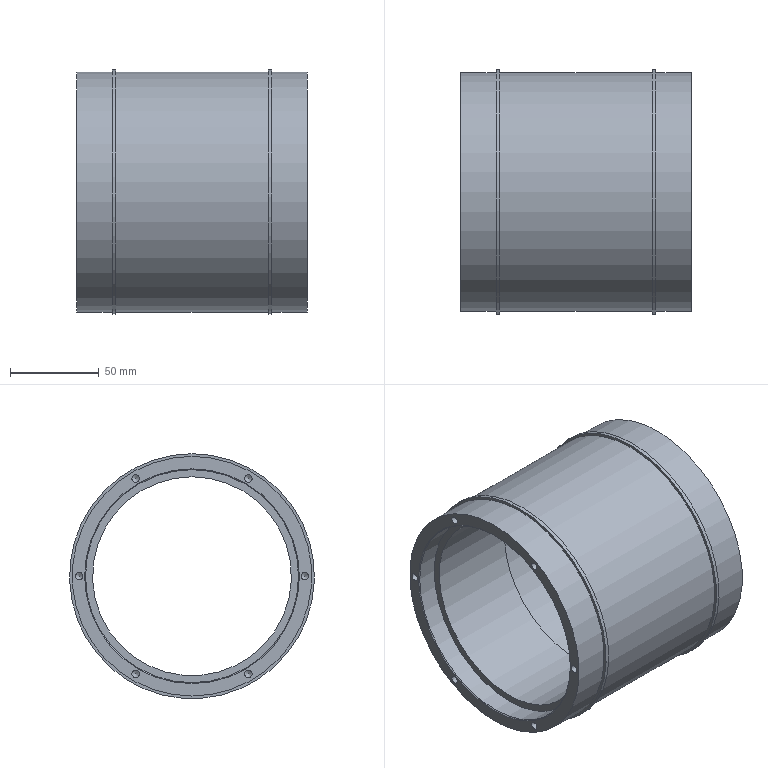Part | NX | features BREP 1 | 1 solid | 44 faces | box 130 x 138 x 138 mm | volume 471054 mm3 | cylinder 21 | cone 14 | plane 9 | commonest cylinder face diameters 4.2 x12 135 x3 120 x2 138 x2 112 x1 119 x1
STEP:
#1=CARTESIAN_POINT('',(-1.085,0.,-60.5));
#2=VERTEX_POINT('',#1);
#3=CARTESIAN_POINT('',(-1.085,0.,0.));
#4=DIRECTION('',(1.,0.,0.));
#5=DIRECTION('',(0.,0.,-1.));
#6=AXIS2_PLACEMENT_3D('',#3,#4,#5);
#7=CIRCLE('',#6,60.5);
#8=EDGE_CURVE('',#2,#2,#7,.T.);
#9=ORIENTED_EDGE('',*,*,#8,.F.);
#10=EDGE_LOOP('',(#9));
#11=FACE_BOUND('',#10,.T.);
#12=CARTESIAN_POINT('',(-0.5854,0.,-60.));
#13=VERTEX_POINT('',#12);
#14=CARTESIAN_POINT('',(-0.5854,0.,0.));
#15=DIRECTION('',(-1.,0.,0.));
#16=DIRECTION('',(0.,0.,-1.));
#17=AXIS2_PLACEMENT_3D('',#14,#15,#16);
#18=CIRCLE('',#17,60.);
#19=EDGE_CURVE('',#13,#13,#18,.T.);
#20=ORIENTED_EDGE('',*,*,#19,.F.);
#21=EDGE_LOOP('',(#20));
#22=FACE_BOUND('',#21,.T.);
#23=CARTESIAN_POINT('',(-0.5854,0.,0.));
#24=DIRECTION('',(-1.,0.,0.));
#25=DIRECTION('',(0.,0.,1.));
#26=AXIS2_PLACEMENT_3D('',#23,#24,#25);
#27=CONICAL_SURFACE('',#26,60.,0.7854);
#28=ADVANCED_FACE('',(#11,#22),#27,.F.);
#29=CARTESIAN_POINT('',(128.915,0.,60.5));
#30=VERTEX_POINT('',#29);
#31=CARTESIAN_POINT('',(128.915,0.,0.));
#32=DIRECTION('',(-1.,0.,0.));
#33=DIRECTION('',(0.,0.,1.));
#34=AXIS2_PLACEMENT_3D('',#31,#32,#33);
#35=CIRCLE('',#34,60.5);
#36=EDGE_CURVE('',#30,#30,#35,.T.);
#37=ORIENTED_EDGE('',*,*,#36,.F.);
#38=EDGE_LOOP('',(#37));
#39=FACE_BOUND('',#38,.T.);
#40=CARTESIAN_POINT('',(128.415,0.,60.));
#41=VERTEX_POINT('',#40);
#42=CARTESIAN_POINT('',(128.415,0.,0.));
#43=DIRECTION('',(1.,0.,0.));
#44=DIRECTION('',(0.,0.,1.));
#45=AXIS2_PLACEMENT_3D('',#42,#43,#44);
#46=CIRCLE('',#45,60.);
#47=EDGE_CURVE('',#41,#41,#46,.T.);
#48=ORIENTED_EDGE('',*,*,#47,.F.);
#49=EDGE_LOOP('',(#48));
#50=FACE_BOUND('',#49,.T.);
#51=CARTESIAN_POINT('',(128.415,0.,0.));
#52=DIRECTION('',(1.,0.,0.));
#53=DIRECTION('',(0.,0.,-1.));
#54=AXIS2_PLACEMENT_3D('',#51,#52,#53);
#55=CONICAL_SURFACE('',#54,60.,0.7854);
#56=ADVANCED_FACE('',(#39,#50),#55,.F.);
#57=ORIENTED_EDGE('',*,*,#47,.T.);
#58=EDGE_LOOP('',(#57));
#59=FACE_BOUND('',#58,.T.);
#60=CARTESIAN_POINT('',(92.915,0.,-60.));
#61=VERTEX_POINT('',#60);
#62=CARTESIAN_POINT('',(92.915,0.,0.));
#63=DIRECTION('',(1.,0.,0.));
#64=DIRECTION('',(0.,0.,-1.));
#65=AXIS2_PLACEMENT_3D('',#62,#63,#64);
#66=CIRCLE('',#65,60.);
#67=EDGE_CURVE('',#61,#61,#66,.T.);
#68=ORIENTED_EDGE('',*,*,#67,.F.);
#69=EDGE_LOOP('',(#68));
#70=FACE_BOUND('',#69,.T.);
#71=CARTESIAN_POINT('',(92.915,0.,0.));
#72=DIRECTION('',(1.,0.,0.));
#73=DIRECTION('',(0.,0.,-1.));
#74=AXIS2_PLACEMENT_3D('',#71,#72,#73);
#75=CYLINDRICAL_SURFACE('',#74,60.);
#76=ADVANCED_FACE('',(#59,#70),#75,.F.);
#77=CARTESIAN_POINT('',(-1.085,31.75,57.093));
#78=VERTEX_POINT('',#77);
#79=CARTESIAN_POINT('',(-1.085,31.75,54.993));
#80=DIRECTION('',(-1.,0.,0.));
#81=DIRECTION('',(0.,0.,1.));
#82=AXIS2_PLACEMENT_3D('',#79,#80,#81);
#83=CIRCLE('',#82,2.1);
#84=EDGE_CURVE('',#78,#78,#83,.T.);
#85=ORIENTED_EDGE('',*,*,#84,.T.);
#86=EDGE_LOOP('',(#85));
#87=FACE_BOUND('',#86,.T.);
#88=CARTESIAN_POINT('',(18.915,31.75,57.093));
#89=VERTEX_POINT('',#88);
#90=CARTESIAN_POINT('',(18.915,31.75,54.993));
#91=DIRECTION('',(-1.,0.,0.));
#92=DIRECTION('',(0.,0.,1.));
#93=AXIS2_PLACEMENT_3D('',#90,#91,#92);
#94=CIRCLE('',#93,2.1);
#95=EDGE_CURVE('',#89,#89,#94,.T.);
#96=ORIENTED_EDGE('',*,*,#95,.F.);
#97=EDGE_LOOP('',(#96));
#98=FACE_BOUND('',#97,.T.);
#99=CARTESIAN_POINT('',(-1.085,31.75,54.993));
#100=DIRECTION('',(-1.,0.,0.));
#101=DIRECTION('',(0.,0.,1.));
#102=AXIS2_PLACEMENT_3D('',#99,#100,#101);
#103=CYLINDRICAL_SURFACE('',#102,2.1);
#104=ADVANCED_FACE('',(#87,#98),#103,.F.);
#105=ORIENTED_EDGE('',*,*,#95,.T.);
#106=EDGE_LOOP('',(#105));
#107=FACE_BOUND('',#106,.T.);
#108=CARTESIAN_POINT('',(20.176,31.75,54.993));
#109=VERTEX_POINT('',#108);
#110=VERTEX_LOOP('',#109);
#111=FACE_BOUND('',#110,.T.);
#112=CARTESIAN_POINT('',(18.915,31.75,54.993));
#113=DIRECTION('',(-1.,0.,0.));
#114=DIRECTION('',(0.,0.,1.));
#115=AXIS2_PLACEMENT_3D('',#112,#113,#114);
#116=CONICAL_SURFACE('',#115,2.1,1.03);
#117=ADVANCED_FACE('',(#107,#111),#116,.F.);
#118=CARTESIAN_POINT('',(-1.085,-31.75,57.093));
#119=VERTEX_POINT('',#118);
#120=CARTESIAN_POINT('',(-1.085,-31.75,54.993));
#121=DIRECTION('',(-1.,0.,0.));
#122=DIRECTION('',(0.,0.,1.));
#123=AXIS2_PLACEMENT_3D('',#120,#121,#122);
#124=CIRCLE('',#123,2.1);
#125=EDGE_CURVE('',#119,#119,#124,.T.);
#126=ORIENTED_EDGE('',*,*,#125,.T.);
#127=EDGE_LOOP('',(#126));
#128=FACE_BOUND('',#127,.T.);
#129=CARTESIAN_POINT('',(18.915,-31.75,57.093));
#130=VERTEX_POINT('',#129);
#131=CARTESIAN_POINT('',(18.915,-31.75,54.993));
#132=DIRECTION('',(-1.,0.,0.));
#133=DIRECTION('',(0.,0.,1.));
#134=AXIS2_PLACEMENT_3D('',#131,#132,#133);
#135=CIRCLE('',#134,2.1);
#136=EDGE_CURVE('',#130,#130,#135,.T.);
#137=ORIENTED_EDGE('',*,*,#136,.F.);
#138=EDGE_LOOP('',(#137));
#139=FACE_BOUND('',#138,.T.);
#140=CARTESIAN_POINT('',(-1.085,-31.75,54.993));
#141=DIRECTION('',(-1.,0.,0.));
#142=DIRECTION('',(0.,0.,1.));
#143=AXIS2_PLACEMENT_3D('',#140,#141,#142);
#144=CYLINDRICAL_SURFACE('',#143,2.1);
#145=ADVANCED_FACE('',(#128,#139),#144,.F.);
#146=ORIENTED_EDGE('',*,*,#136,.T.);
#147=EDGE_LOOP('',(#146));
#148=FACE_BOUND('',#147,.T.);
#149=CARTESIAN_POINT('',(20.176,-31.75,54.993));
#150=VERTEX_POINT('',#149);
#151=VERTEX_LOOP('',#150);
#152=FACE_BOUND('',#151,.T.);
#153=CARTESIAN_POINT('',(18.915,-31.75,54.993));
#154=DIRECTION('',(-1.,0.,0.));
#155=DIRECTION('',(0.,0.,1.));
#156=AXIS2_PLACEMENT_3D('',#153,#154,#155);
#157=CONICAL_SURFACE('',#156,2.1,1.03);
#158=ADVANCED_FACE('',(#148,#152),#157,.F.);
#159=CARTESIAN_POINT('',(-1.085,-63.5,2.1));
#160=VERTEX_POINT('',#159);
#161=CARTESIAN_POINT('',(-1.085,-63.5,0.));
#162=DIRECTION('',(-1.,0.,0.));
#163=DIRECTION('',(0.,0.,1.));
#164=AXIS2_PLACEMENT_3D('',#161,#162,#163);
#165=CIRCLE('',#164,2.1);
#166=EDGE_CURVE('',#160,#160,#165,.T.);
#167=ORIENTED_EDGE('',*,*,#166,.T.);
#168=EDGE_LOOP('',(#167));
#169=FACE_BOUND('',#168,.T.);
#170=CARTESIAN_POINT('',(18.915,-63.5,2.1));
#171=VERTEX_POINT('',#170);
#172=CARTESIAN_POINT('',(18.915,-63.5,0.));
#173=DIRECTION('',(-1.,0.,0.));
#174=DIRECTION('',(0.,0.,1.));
#175=AXIS2_PLACEMENT_3D('',#172,#173,#174);
#176=CIRCLE('',#175,2.1);
#177=EDGE_CURVE('',#171,#171,#176,.T.);
#178=ORIENTED_EDGE('',*,*,#177,.F.);
#179=EDGE_LOOP('',(#178));
#180=FACE_BOUND('',#179,.T.);
#181=CARTESIAN_POINT('',(-1.085,-63.5,0.));
#182=DIRECTION('',(-1.,0.,0.));
#183=DIRECTION('',(0.,0.,1.));
#184=AXIS2_PLACEMENT_3D('',#181,#182,#183);
#185=CYLINDRICAL_SURFACE('',#184,2.1);
#186=ADVANCED_FACE('',(#169,#180),#185,.F.);
#187=ORIENTED_EDGE('',*,*,#177,.T.);
#188=EDGE_LOOP('',(#187));
#189=FACE_BOUND('',#188,.T.);
#190=CARTESIAN_POINT('',(20.176,-63.5,0.));
#191=VERTEX_POINT('',#190);
#192=VERTEX_LOOP('',#191);
#193=FACE_BOUND('',#192,.T.);
#194=CARTESIAN_POINT('',(18.915,-63.5,0.));
#195=DIRECTION('',(-1.,0.,0.));
#196=DIRECTION('',(0.,0.,1.));
#197=AXIS2_PLACEMENT_3D('',#194,#195,#196);
#198=CONICAL_SURFACE('',#197,2.1,1.03);
#199=ADVANCED_FACE('',(#189,#193),#198,.F.);
#200=CARTESIAN_POINT('',(-1.085,-31.75,-52.893));
#201=VERTEX_POINT('',#200);
#202=CARTESIAN_POINT('',(-1.085,-31.75,-54.993));
#203=DIRECTION('',(-1.,0.,0.));
#204=DIRECTION('',(0.,0.,1.));
#205=AXIS2_PLACEMENT_3D('',#202,#203,#204);
#206=CIRCLE('',#205,2.1);
#207=EDGE_CURVE('',#201,#201,#206,.T.);
#208=ORIENTED_EDGE('',*,*,#207,.T.);
#209=EDGE_LOOP('',(#208));
#210=FACE_BOUND('',#209,.T.);
#211=CARTESIAN_POINT('',(18.915,-31.75,-52.893));
#212=VERTEX_POINT('',#211);
#213=CARTESIAN_POINT('',(18.915,-31.75,-54.993));
#214=DIRECTION('',(-1.,0.,0.));
#215=DIRECTION('',(0.,0.,1.));
#216=AXIS2_PLACEMENT_3D('',#213,#214,#215);
#217=CIRCLE('',#216,2.1);
#218=EDGE_CURVE('',#212,#212,#217,.T.);
#219=ORIENTED_EDGE('',*,*,#218,.F.);
#220=EDGE_LOOP('',(#219));
#221=FACE_BOUND('',#220,.T.);
#222=CARTESIAN_POINT('',(-1.085,-31.75,-54.993));
#223=DIRECTION('',(-1.,0.,0.));
#224=DIRECTION('',(0.,0.,1.));
#225=AXIS2_PLACEMENT_3D('',#222,#223,#224);
#226=CYLINDRICAL_SURFACE('',#225,2.1);
#227=ADVANCED_FACE('',(#210,#221),#226,.F.);
#228=ORIENTED_EDGE('',*,*,#218,.T.);
#229=EDGE_LOOP('',(#228));
#230=FACE_BOUND('',#229,.T.);
#231=CARTESIAN_POINT('',(20.176,-31.75,-54.993));
#232=VERTEX_POINT('',#231);
#233=VERTEX_LOOP('',#232);
#234=FACE_BOUND('',#233,.T.);
#235=CARTESIAN_POINT('',(18.915,-31.75,-54.993));
#236=DIRECTION('',(-1.,0.,0.));
#237=DIRECTION('',(0.,0.,1.));
#238=AXIS2_PLACEMENT_3D('',#235,#236,#237);
#239=CONICAL_SURFACE('',#238,2.1,1.03);
#240=ADVANCED_FACE('',(#230,#234),#239,.F.);
#241=CARTESIAN_POINT('',(-1.085,31.75,-52.893));
#242=VERTEX_POINT('',#241);
#243=CARTESIAN_POINT('',(-1.085,31.75,-54.993));
#244=DIRECTION('',(-1.,0.,0.));
#245=DIRECTION('',(0.,0.,1.));
#246=AXIS2_PLACEMENT_3D('',#243,#244,#245);
#247=CIRCLE('',#246,2.1);
#248=EDGE_CURVE('',#242,#242,#247,.T.);
#249=ORIENTED_EDGE('',*,*,#248,.T.);
#250=EDGE_LOOP('',(#249));
#251=FACE_BOUND('',#250,.T.);
#252=CARTESIAN_POINT('',(18.915,31.75,-52.893));
#253=VERTEX_POINT('',#252);
#254=CARTESIAN_POINT('',(18.915,31.75,-54.993));
#255=DIRECTION('',(-1.,0.,0.));
#256=DIRECTION('',(0.,0.,1.));
#257=AXIS2_PLACEMENT_3D('',#254,#255,#256);
#258=CIRCLE('',#257,2.1);
#259=EDGE_CURVE('',#253,#253,#258,.T.);
#260=ORIENTED_EDGE('',*,*,#259,.F.);
#261=EDGE_LOOP('',(#260));
#262=FACE_BOUND('',#261,.T.);
#263=CARTESIAN_POINT('',(-1.085,31.75,-54.993));
#264=DIRECTION('',(-1.,0.,0.));
#265=DIRECTION('',(0.,0.,1.));
#266=AXIS2_PLACEMENT_3D('',#263,#264,#265);
#267=CYLINDRICAL_SURFACE('',#266,2.1);
#268=ADVANCED_FACE('',(#251,#262),#267,.F.);
#269=ORIENTED_EDGE('',*,*,#259,.T.);
#270=EDGE_LOOP('',(#269));
#271=FACE_BOUND('',#270,.T.);
#272=CARTESIAN_POINT('',(20.176,31.75,-54.993));
#273=VERTEX_POINT('',#272);
#274=VERTEX_LOOP('',#273);
#275=FACE_BOUND('',#274,.T.);
#276=CARTESIAN_POINT('',(18.915,31.75,-54.993));
#277=DIRECTION('',(-1.,0.,0.));
#278=DIRECTION('',(0.,0.,1.));
#279=AXIS2_PLACEMENT_3D('',#276,#277,#278);
#280=CONICAL_SURFACE('',#279,2.1,1.03);
#281=ADVANCED_FACE('',(#271,#275),#280,.F.);
#282=CARTESIAN_POINT('',(-1.085,63.5,2.1));
#283=VERTEX_POINT('',#282);
#284=CARTESIAN_POINT('',(-1.085,63.5,0.));
#285=DIRECTION('',(-1.,0.,0.));
#286=DIRECTION('',(0.,0.,1.));
#287=AXIS2_PLACEMENT_3D('',#284,#285,#286);
#288=CIRCLE('',#287,2.1);
#289=EDGE_CURVE('',#283,#283,#288,.T.);
#290=ORIENTED_EDGE('',*,*,#289,.T.);
#291=EDGE_LOOP('',(#290));
#292=FACE_BOUND('',#291,.T.);
#293=CARTESIAN_POINT('',(18.915,63.5,2.1));
#294=VERTEX_POINT('',#293);
#295=CARTESIAN_POINT('',(18.915,63.5,0.));
#296=DIRECTION('',(-1.,0.,0.));
#297=DIRECTION('',(0.,0.,1.));
#298=AXIS2_PLACEMENT_3D('',#295,#296,#297);
#299=CIRCLE('',#298,2.1);
#300=EDGE_CURVE('',#294,#294,#299,.T.);
#301=ORIENTED_EDGE('',*,*,#300,.F.);
#302=EDGE_LOOP('',(#301));
#303=FACE_BOUND('',#302,.T.);
#304=CARTESIAN_POINT('',(-1.085,63.5,0.));
#305=DIRECTION('',(-1.,0.,0.));
#306=DIRECTION('',(0.,0.,1.));
#307=AXIS2_PLACEMENT_3D('',#304,#305,#306);
#308=CYLINDRICAL_SURFACE('',#307,2.1);
#309=ADVANCED_FACE('',(#292,#303),#308,.F.);
#310=ORIENTED_EDGE('',*,*,#300,.T.);
#311=EDGE_LOOP('',(#310));
#312=FACE_BOUND('',#311,.T.);
#313=CARTESIAN_POINT('',(20.176,63.5,0.));
#314=VERTEX_POINT('',#313);
#315=VERTEX_LOOP('',#314);
#316=FACE_BOUND('',#315,.T.);
#317=CARTESIAN_POINT('',(18.915,63.5,0.));
#318=DIRECTION('',(-1.,0.,0.));
#319=DIRECTION('',(0.,0.,1.));
#320=AXIS2_PLACEMENT_3D('',#317,#318,#319);
#321=CONICAL_SURFACE('',#320,2.1,1.03);
#322=ADVANCED_FACE('',(#312,#316),#321,.F.);
#323=CARTESIAN_POINT('',(128.915,31.75,52.893));
#324=VERTEX_POINT('',#323);
#325=CARTESIAN_POINT('',(128.915,31.75,54.993));
#326=DIRECTION('',(1.,0.,0.));
#327=DIRECTION('',(0.,0.,-1.));
#328=AXIS2_PLACEMENT_3D('',#325,#326,#327);
#329=CIRCLE('',#328,2.1);
#330=EDGE_CURVE('',#324,#324,#329,.T.);
#331=ORIENTED_EDGE('',*,*,#330,.T.);
#332=EDGE_LOOP('',(#331));
#333=FACE_BOUND('',#332,.T.);
#334=CARTESIAN_POINT('',(108.915,31.75,52.893));
#335=VERTEX_POINT('',#334);
#336=CARTESIAN_POINT('',(108.915,31.75,54.993));
#337=DIRECTION('',(1.,0.,0.));
#338=DIRECTION('',(0.,0.,-1.));
#339=AXIS2_PLACEMENT_3D('',#336,#337,#338);
#340=CIRCLE('',#339,2.1);
#341=EDGE_CURVE('',#335,#335,#340,.T.);
#342=ORIENTED_EDGE('',*,*,#341,.F.);
#343=EDGE_LOOP('',(#342));
#344=FACE_BOUND('',#343,.T.);
#345=CARTESIAN_POINT('',(128.915,31.75,54.993));
#346=DIRECTION('',(1.,0.,0.));
#347=DIRECTION('',(0.,0.,-1.));
#348=AXIS2_PLACEMENT_3D('',#345,#346,#347);
#349=CYLINDRICAL_SURFACE('',#348,2.1);
#350=ADVANCED_FACE('',(#333,#344),#349,.F.);
#351=ORIENTED_EDGE('',*,*,#341,.T.);
#352=EDGE_LOOP('',(#351));
#353=FACE_BOUND('',#352,.T.);
#354=CARTESIAN_POINT('',(107.653,31.75,54.993));
#355=VERTEX_POINT('',#354);
#356=VERTEX_LOOP('',#355);
#357=FACE_BOUND('',#356,.T.);
#358=CARTESIAN_POINT('',(108.915,31.75,54.993));
#359=DIRECTION('',(1.,0.,0.));
#360=DIRECTION('',(0.,0.,-1.));
#361=AXIS2_PLACEMENT_3D('',#358,#359,#360);
#362=CONICAL_SURFACE('',#361,2.1,1.03);
#363=ADVANCED_FACE('',(#353,#357),#362,.F.);
#364=CARTESIAN_POINT('',(128.915,-31.75,52.893));
#365=VERTEX_POINT('',#364);
#366=CARTESIAN_POINT('',(128.915,-31.75,54.993));
#367=DIRECTION('',(1.,0.,0.));
#368=DIRECTION('',(0.,0.,-1.));
#369=AXIS2_PLACEMENT_3D('',#366,#367,#368);
#370=CIRCLE('',#369,2.1);
#371=EDGE_CURVE('',#365,#365,#370,.T.);
#372=ORIENTED_EDGE('',*,*,#371,.T.);
#373=EDGE_LOOP('',(#372));
#374=FACE_BOUND('',#373,.T.);
#375=CARTESIAN_POINT('',(108.915,-31.75,52.893));
#376=VERTEX_POINT('',#375);
#377=CARTESIAN_POINT('',(108.915,-31.75,54.993));
#378=DIRECTION('',(1.,0.,0.));
#379=DIRECTION('',(0.,0.,-1.));
#380=AXIS2_PLACEMENT_3D('',#377,#378,#379);
#381=CIRCLE('',#380,2.1);
#382=EDGE_CURVE('',#376,#376,#381,.T.);
#383=ORIENTED_EDGE('',*,*,#382,.F.);
#384=EDGE_LOOP('',(#383));
#385=FACE_BOUND('',#384,.T.);
#386=CARTESIAN_POINT('',(128.915,-31.75,54.993));
#387=DIRECTION('',(1.,0.,0.));
#388=DIRECTION('',(0.,0.,-1.));
#389=AXIS2_PLACEMENT_3D('',#386,#387,#388);
#390=CYLINDRICAL_SURFACE('',#389,2.1);
#391=ADVANCED_FACE('',(#374,#385),#390,.F.);
#392=ORIENTED_EDGE('',*,*,#382,.T.);
#393=EDGE_LOOP('',(#392));
#394=FACE_BOUND('',#393,.T.);
#395=CARTESIAN_POINT('',(107.653,-31.75,54.993));
#396=VERTEX_POINT('',#395);
#397=VERTEX_LOOP('',#396);
#398=FACE_BOUND('',#397,.T.);
#399=CARTESIAN_POINT('',(108.915,-31.75,54.993));
#400=DIRECTION('',(1.,0.,0.));
#401=DIRECTION('',(0.,0.,-1.));
#402=AXIS2_PLACEMENT_3D('',#399,#400,#401);
#403=CONICAL_SURFACE('',#402,2.1,1.03);
#404=ADVANCED_FACE('',(#394,#398),#403,.F.);
#405=CARTESIAN_POINT('',(128.915,-63.5,-2.1));
#406=VERTEX_POINT('',#405);
#407=CARTESIAN_POINT('',(128.915,-63.5,0.));
#408=DIRECTION('',(1.,0.,0.));
#409=DIRECTION('',(0.,0.,-1.));
#410=AXIS2_PLACEMENT_3D('',#407,#408,#409);
#411=CIRCLE('',#410,2.1);
#412=EDGE_CURVE('',#406,#406,#411,.T.);
#413=ORIENTED_EDGE('',*,*,#412,.T.);
#414=EDGE_LOOP('',(#413));
#415=FACE_BOUND('',#414,.T.);
#416=CARTESIAN_POINT('',(108.915,-63.5,-2.1));
#417=VERTEX_POINT('',#416);
#418=CARTESIAN_POINT('',(108.915,-63.5,0.));
#419=DIRECTION('',(1.,0.,0.));
#420=DIRECTION('',(0.,0.,-1.));
#421=AXIS2_PLACEMENT_3D('',#418,#419,#420);
#422=CIRCLE('',#421,2.1);
#423=EDGE_CURVE('',#417,#417,#422,.T.);
#424=ORIENTED_EDGE('',*,*,#423,.F.);
#425=EDGE_LOOP('',(#424));
#426=FACE_BOUND('',#425,.T.);
#427=CARTESIAN_POINT('',(128.915,-63.5,0.));
#428=DIRECTION('',(1.,0.,0.));
#429=DIRECTION('',(0.,0.,-1.));
#430=AXIS2_PLACEMENT_3D('',#427,#428,#429);
#431=CYLINDRICAL_SURFACE('',#430,2.1);
#432=ADVANCED_FACE('',(#415,#426),#431,.F.);
#433=ORIENTED_EDGE('',*,*,#423,.T.);
#434=EDGE_LOOP('',(#433));
#435=FACE_BOUND('',#434,.T.);
#436=CARTESIAN_POINT('',(107.653,-63.5,0.));
#437=VERTEX_POINT('',#436);
#438=VERTEX_LOOP('',#437);
#439=FACE_BOUND('',#438,.T.);
#440=CARTESIAN_POINT('',(108.915,-63.5,0.));
#441=DIRECTION('',(1.,0.,0.));
#442=DIRECTION('',(0.,0.,-1.));
#443=AXIS2_PLACEMENT_3D('',#440,#441,#442);
#444=CONICAL_SURFACE('',#443,2.1,1.03);
#445=ADVANCED_FACE('',(#435,#439),#444,.F.);
#446=CARTESIAN_POINT('',(128.915,-31.75,-57.093));
#447=VERTEX_POINT('',#446);
#448=CARTESIAN_POINT('',(128.915,-31.75,-54.993));
#449=DIRECTION('',(1.,0.,0.));
#450=DIRECTION('',(0.,0.,-1.));
#451=AXIS2_PLACEMENT_3D('',#448,#449,#450);
#452=CIRCLE('',#451,2.1);
#453=EDGE_CURVE('',#447,#447,#452,.T.);
#454=ORIENTED_EDGE('',*,*,#453,.T.);
#455=EDGE_LOOP('',(#454));
#456=FACE_BOUND('',#455,.T.);
#457=CARTESIAN_POINT('',(108.915,-31.75,-57.093));
#458=VERTEX_POINT('',#457);
#459=CARTESIAN_POINT('',(108.915,-31.75,-54.993));
#460=DIRECTION('',(1.,0.,0.));
#461=DIRECTION('',(0.,0.,-1.));
#462=AXIS2_PLACEMENT_3D('',#459,#460,#461);
#463=CIRCLE('',#462,2.1);
#464=EDGE_CURVE('',#458,#458,#463,.T.);
#465=ORIENTED_EDGE('',*,*,#464,.F.);
#466=EDGE_LOOP('',(#465));
#467=FACE_BOUND('',#466,.T.);
#468=CARTESIAN_POINT('',(128.915,-31.75,-54.993));
#469=DIRECTION('',(1.,0.,0.));
#470=DIRECTION('',(0.,0.,-1.));
#471=AXIS2_PLACEMENT_3D('',#468,#469,#470);
#472=CYLINDRICAL_SURFACE('',#471,2.1);
#473=ADVANCED_FACE('',(#456,#467),#472,.F.);
#474=ORIENTED_EDGE('',*,*,#464,.T.);
#475=EDGE_LOOP('',(#474));
#476=FACE_BOUND('',#475,.T.);
#477=CARTESIAN_POINT('',(107.653,-31.75,-54.993));
#478=VERTEX_POINT('',#477);
#479=VERTEX_LOOP('',#478);
#480=FACE_BOUND('',#479,.T.);
#481=CARTESIAN_POINT('',(108.915,-31.75,-54.993));
#482=DIRECTION('',(1.,0.,0.));
#483=DIRECTION('',(0.,0.,-1.));
#484=AXIS2_PLACEMENT_3D('',#481,#482,#483);
#485=CONICAL_SURFACE('',#484,2.1,1.03);
#486=ADVANCED_FACE('',(#476,#480),#485,.F.);
#487=CARTESIAN_POINT('',(128.915,31.75,-57.093));
#488=VERTEX_POINT('',#487);
#489=CARTESIAN_POINT('',(128.915,31.75,-54.993));
#490=DIRECTION('',(1.,0.,0.));
#491=DIRECTION('',(0.,0.,-1.));
#492=AXIS2_PLACEMENT_3D('',#489,#490,#491);
#493=CIRCLE('',#492,2.1);
#494=EDGE_CURVE('',#488,#488,#493,.T.);
#495=ORIENTED_EDGE('',*,*,#494,.T.);
#496=EDGE_LOOP('',(#495));
#497=FACE_BOUND('',#496,.T.);
#498=CARTESIAN_POINT('',(108.915,31.75,-57.093));
#499=VERTEX_POINT('',#498);
#500=CARTESIAN_POINT('',(108.915,31.75,-54.993));
#501=DIRECTION('',(1.,0.,0.));
#502=DIRECTION('',(0.,0.,-1.));
#503=AXIS2_PLACEMENT_3D('',#500,#501,#502);
#504=CIRCLE('',#503,2.1);
#505=EDGE_CURVE('',#499,#499,#504,.T.);
#506=ORIENTED_EDGE('',*,*,#505,.F.);
#507=EDGE_LOOP('',(#506));
#508=FACE_BOUND('',#507,.T.);
#509=CARTESIAN_POINT('',(128.915,31.75,-54.993));
#510=DIRECTION('',(1.,0.,0.));
#511=DIRECTION('',(0.,0.,-1.));
#512=AXIS2_PLACEMENT_3D('',#509,#510,#511);
#513=CYLINDRICAL_SURFACE('',#512,2.1);
#514=ADVANCED_FACE('',(#497,#508),#513,.F.);
#515=ORIENTED_EDGE('',*,*,#505,.T.);
#516=EDGE_LOOP('',(#515));
#517=FACE_BOUND('',#516,.T.);
#518=CARTESIAN_POINT('',(107.653,31.75,-54.993));
#519=VERTEX_POINT('',#518);
#520=VERTEX_LOOP('',#519);
#521=FACE_BOUND('',#520,.T.);
#522=CARTESIAN_POINT('',(108.915,31.75,-54.993));
#523=DIRECTION('',(1.,0.,0.));
#524=DIRECTION('',(0.,0.,-1.));
#525=AXIS2_PLACEMENT_3D('',#522,#523,#524);
#526=CONICAL_SURFACE('',#525,2.1,1.03);
#527=ADVANCED_FACE('',(#517,#521),#526,.F.);
#528=CARTESIAN_POINT('',(128.915,63.5,-2.1));
#529=VERTEX_POINT('',#528);
#530=CARTESIAN_POINT('',(128.915,63.5,0.));
#531=DIRECTION('',(1.,0.,0.));
#532=DIRECTION('',(0.,0.,-1.));
#533=AXIS2_PLACEMENT_3D('',#530,#531,#532);
#534=CIRCLE('',#533,2.1);
#535=EDGE_CURVE('',#529,#529,#534,.T.);
#536=ORIENTED_EDGE('',*,*,#535,.T.);
#537=EDGE_LOOP('',(#536));
#538=FACE_BOUND('',#537,.T.);
#539=CARTESIAN_POINT('',(108.915,63.5,-2.1));
#540=VERTEX_POINT('',#539);
#541=CARTESIAN_POINT('',(108.915,63.5,0.));
#542=DIRECTION('',(1.,0.,0.));
#543=DIRECTION('',(0.,0.,-1.));
#544=AXIS2_PLACEMENT_3D('',#541,#542,#543);
#545=CIRCLE('',#544,2.1);
#546=EDGE_CURVE('',#540,#540,#545,.T.);
#547=ORIENTED_EDGE('',*,*,#546,.F.);
#548=EDGE_LOOP('',(#547));
#549=FACE_BOUND('',#548,.T.);
#550=CARTESIAN_POINT('',(128.915,63.5,0.));
#551=DIRECTION('',(1.,0.,0.));
#552=DIRECTION('',(0.,0.,-1.));
#553=AXIS2_PLACEMENT_3D('',#550,#551,#552);
#554=CYLINDRICAL_SURFACE('',#553,2.1);
#555=ADVANCED_FACE('',(#538,#549),#554,.F.);
#556=ORIENTED_EDGE('',*,*,#546,.T.);
#557=EDGE_LOOP('',(#556));
#558=FACE_BOUND('',#557,.T.);
#559=CARTESIAN_POINT('',(107.653,63.5,0.));
#560=VERTEX_POINT('',#559);
#561=VERTEX_LOOP('',#560);
#562=FACE_BOUND('',#561,.T.);
#563=CARTESIAN_POINT('',(108.915,63.5,0.));
#564=DIRECTION('',(1.,0.,0.));
#565=DIRECTION('',(0.,0.,-1.));
#566=AXIS2_PLACEMENT_3D('',#563,#564,#565);
#567=CONICAL_SURFACE('',#566,2.1,1.03);
#568=ADVANCED_FACE('',(#558,#562),#567,.F.);
#569=CARTESIAN_POINT('',(-1.085,0.,67.5));
#570=VERTEX_POINT('',#569);
#571=CARTESIAN_POINT('',(-1.085,0.,0.));
#572=DIRECTION('',(-1.,0.,0.));
#573=DIRECTION('',(0.,0.,1.));
#574=AXIS2_PLACEMENT_3D('',#571,#572,#573);
#575=CIRCLE('',#574,67.5);
#576=EDGE_CURVE('',#570,#570,#575,.T.);
#577=ORIENTED_EDGE('',*,*,#576,.F.);
#578=EDGE_LOOP('',(#577));
#579=FACE_BOUND('',#578,.T.);
#580=CARTESIAN_POINT('',(18.915,0.,67.5));
#581=VERTEX_POINT('',#580);
#582=CARTESIAN_POINT('',(18.915,0.,0.));
#583=DIRECTION('',(-1.,0.,0.));
#584=DIRECTION('',(0.,0.,1.));
#585=AXIS2_PLACEMENT_3D('',#582,#583,#584);
#586=CIRCLE('',#585,67.5);
#587=EDGE_CURVE('',#581,#581,#586,.T.);
#588=ORIENTED_EDGE('',*,*,#587,.T.);
#589=EDGE_LOOP('',(#588));
#590=FACE_BOUND('',#589,.T.);
#591=CARTESIAN_POINT('',(0.,0.,0.));
#592=DIRECTION('',(-1.,0.,0.));
#593=DIRECTION('',(0.,0.,1.));
#594=AXIS2_PLACEMENT_3D('',#591,#592,#593);
#595=CYLINDRICAL_SURFACE('',#594,67.5);
#596=ADVANCED_FACE('',(#579,#590),#595,.T.);
#597=CARTESIAN_POINT('',(18.915,0.,69.));
#598=VERTEX_POINT('',#597);
#599=CARTESIAN_POINT('',(18.915,0.,0.));
#600=DIRECTION('',(-1.,0.,0.));
#601=DIRECTION('',(0.,0.,1.));
#602=AXIS2_PLACEMENT_3D('',#599,#600,#601);
#603=CIRCLE('',#602,69.);
#604=EDGE_CURVE('',#598,#598,#603,.T.);
#605=ORIENTED_EDGE('',*,*,#604,.F.);
#606=EDGE_LOOP('',(#605));
#607=FACE_BOUND('',#606,.T.);
#608=CARTESIAN_POINT('',(20.915,0.,69.));
#609=VERTEX_POINT('',#608);
#610=CARTESIAN_POINT('',(20.915,0.,0.));
#611=DIRECTION('',(-1.,0.,0.));
#612=DIRECTION('',(0.,0.,1.));
#613=AXIS2_PLACEMENT_3D('',#610,#611,#612);
#614=CIRCLE('',#613,69.);
#615=EDGE_CURVE('',#609,#609,#614,.T.);
#616=ORIENTED_EDGE('',*,*,#615,.T.);
#617=EDGE_LOOP('',(#616));
#618=FACE_BOUND('',#617,.T.);
#619=CARTESIAN_POINT('',(0.,0.,0.));
#620=DIRECTION('',(-1.,0.,0.));
#621=DIRECTION('',(0.,0.,1.));
#622=AXIS2_PLACEMENT_3D('',#619,#620,#621);
#623=CYLINDRICAL_SURFACE('',#622,69.);
#624=ADVANCED_FACE('',(#607,#618),#623,.T.);
#625=CARTESIAN_POINT('',(20.915,0.,67.5));
#626=VERTEX_POINT('',#625);
#627=CARTESIAN_POINT('',(20.915,0.,0.));
#628=DIRECTION('',(-1.,0.,0.));
#629=DIRECTION('',(0.,0.,1.));
#630=AXIS2_PLACEMENT_3D('',#627,#628,#629);
#631=CIRCLE('',#630,67.5);
#632=EDGE_CURVE('',#626,#626,#631,.T.);
#633=ORIENTED_EDGE('',*,*,#632,.F.);
#634=EDGE_LOOP('',(#633));
#635=FACE_BOUND('',#634,.T.);
#636=CARTESIAN_POINT('',(106.915,0.,67.5));
#637=VERTEX_POINT('',#636);
#638=CARTESIAN_POINT('',(106.915,0.,0.));
#639=DIRECTION('',(-1.,0.,0.));
#640=DIRECTION('',(0.,0.,1.));
#641=AXIS2_PLACEMENT_3D('',#638,#639,#640);
#642=CIRCLE('',#641,67.5);
#643=EDGE_CURVE('',#637,#637,#642,.T.);
#644=ORIENTED_EDGE('',*,*,#643,.T.);
#645=EDGE_LOOP('',(#644));
#646=FACE_BOUND('',#645,.T.);
#647=CARTESIAN_POINT('',(0.,0.,0.));
#648=DIRECTION('',(-1.,0.,0.));
#649=DIRECTION('',(0.,0.,1.));
#650=AXIS2_PLACEMENT_3D('',#647,#648,#649);
#651=CYLINDRICAL_SURFACE('',#650,67.5);
#652=ADVANCED_FACE('',(#635,#646),#651,.T.);
#653=CARTESIAN_POINT('',(106.915,0.,69.));
#654=VERTEX_POINT('',#653);
#655=CARTESIAN_POINT('',(106.915,0.,0.));
#656=DIRECTION('',(-1.,0.,0.));
#657=DIRECTION('',(0.,0.,1.));
#658=AXIS2_PLACEMENT_3D('',#655,#656,#657);
#659=CIRCLE('',#658,69.);
#660=EDGE_CURVE('',#654,#654,#659,.T.);
#661=ORIENTED_EDGE('',*,*,#660,.F.);
#662=EDGE_LOOP('',(#661));
#663=FACE_BOUND('',#662,.T.);
#664=CARTESIAN_POINT('',(108.915,0.,69.));
#665=VERTEX_POINT('',#664);
#666=CARTESIAN_POINT('',(108.915,0.,0.));
#667=DIRECTION('',(-1.,0.,0.));
#668=DIRECTION('',(0.,0.,1.));
#669=AXIS2_PLACEMENT_3D('',#666,#667,#668);
#670=CIRCLE('',#669,69.);
#671=EDGE_CURVE('',#665,#665,#670,.T.);
#672=ORIENTED_EDGE('',*,*,#671,.T.);
#673=EDGE_LOOP('',(#672));
#674=FACE_BOUND('',#673,.T.);
#675=CARTESIAN_POINT('',(0.,0.,0.));
#676=DIRECTION('',(-1.,0.,0.));
#677=DIRECTION('',(0.,0.,1.));
#678=AXIS2_PLACEMENT_3D('',#675,#676,#677);
#679=CYLINDRICAL_SURFACE('',#678,69.);
#680=ADVANCED_FACE('',(#663,#674),#679,.T.);
#681=CARTESIAN_POINT('',(108.915,0.,67.5));
#682=VERTEX_POINT('',#681);
#683=CARTESIAN_POINT('',(108.915,0.,0.));
#684=DIRECTION('',(-1.,0.,0.));
#685=DIRECTION('',(0.,0.,1.));
#686=AXIS2_PLACEMENT_3D('',#683,#684,#685);
#687=CIRCLE('',#686,67.5);
#688=EDGE_CURVE('',#682,#682,#687,.T.);
#689=ORIENTED_EDGE('',*,*,#688,.F.);
#690=EDGE_LOOP('',(#689));
#691=FACE_BOUND('',#690,.T.);
#692=CARTESIAN_POINT('',(128.915,0.,67.5));
#693=VERTEX_POINT('',#692);
#694=CARTESIAN_POINT('',(128.915,0.,0.));
#695=DIRECTION('',(-1.,0.,0.));
#696=DIRECTION('',(0.,0.,1.));
#697=AXIS2_PLACEMENT_3D('',#694,#695,#696);
#698=CIRCLE('',#697,67.5);
#699=EDGE_CURVE('',#693,#693,#698,.T.);
#700=ORIENTED_EDGE('',*,*,#699,.T.);
#701=EDGE_LOOP('',(#700));
#702=FACE_BOUND('',#701,.T.);
#703=CARTESIAN_POINT('',(0.,0.,0.));
#704=DIRECTION('',(-1.,0.,0.));
#705=DIRECTION('',(0.,0.,1.));
#706=AXIS2_PLACEMENT_3D('',#703,#704,#705);
#707=CYLINDRICAL_SURFACE('',#706,67.5);
#708=ADVANCED_FACE('',(#691,#702),#707,.T.);
#709=CARTESIAN_POINT('',(10.915,0.,56.));
#710=VERTEX_POINT('',#709);
#711=CARTESIAN_POINT('',(10.915,0.,0.));
#712=DIRECTION('',(-1.,0.,0.));
#713=DIRECTION('',(0.,0.,1.));
#714=AXIS2_PLACEMENT_3D('',#711,#712,#713);
#715=CIRCLE('',#714,56.);
#716=EDGE_CURVE('',#710,#710,#715,.T.);
#717=ORIENTED_EDGE('',*,*,#716,.T.);
#718=EDGE_LOOP('',(#717));
#719=FACE_BOUND('',#718,.T.);
#720=CARTESIAN_POINT('',(62.915,0.,56.));
#721=VERTEX_POINT('',#720);
#722=CARTESIAN_POINT('',(62.915,0.,0.));
#723=DIRECTION('',(-1.,0.,0.));
#724=DIRECTION('',(0.,0.,1.));
#725=AXIS2_PLACEMENT_3D('',#722,#723,#724);
#726=CIRCLE('',#725,56.);
#727=EDGE_CURVE('',#721,#721,#726,.T.);
#728=ORIENTED_EDGE('',*,*,#727,.F.);
#729=EDGE_LOOP('',(#728));
#730=FACE_BOUND('',#729,.T.);
#731=CARTESIAN_POINT('',(0.,0.,0.));
#732=DIRECTION('',(-1.,0.,0.));
#733=DIRECTION('',(0.,0.,1.));
#734=AXIS2_PLACEMENT_3D('',#731,#732,#733);
#735=CYLINDRICAL_SURFACE('',#734,56.);
#736=ADVANCED_FACE('',(#719,#730),#735,.F.);
#737=ORIENTED_EDGE('',*,*,#19,.T.);
#738=EDGE_LOOP('',(#737));
#739=FACE_BOUND('',#738,.T.);
#740=CARTESIAN_POINT('',(10.915,0.,60.));
#741=VERTEX_POINT('',#740);
#742=CARTESIAN_POINT('',(10.915,0.,0.));
#743=DIRECTION('',(-1.,0.,0.));
#744=DIRECTION('',(0.,0.,1.));
#745=AXIS2_PLACEMENT_3D('',#742,#743,#744);
#746=CIRCLE('',#745,60.);
#747=EDGE_CURVE('',#741,#741,#746,.T.);
#748=ORIENTED_EDGE('',*,*,#747,.F.);
#749=EDGE_LOOP('',(#748));
#750=FACE_BOUND('',#749,.T.);
#751=CARTESIAN_POINT('',(0.,0.,0.));
#752=DIRECTION('',(-1.,0.,0.));
#753=DIRECTION('',(0.,0.,1.));
#754=AXIS2_PLACEMENT_3D('',#751,#752,#753);
#755=CYLINDRICAL_SURFACE('',#754,60.);
#756=ADVANCED_FACE('',(#739,#750),#755,.F.);
#757=CARTESIAN_POINT('',(62.915,0.,59.5));
#758=VERTEX_POINT('',#757);
#759=CARTESIAN_POINT('',(62.915,0.,0.));
#760=DIRECTION('',(-1.,0.,0.));
#761=DIRECTION('',(0.,0.,1.));
#762=AXIS2_PLACEMENT_3D('',#759,#760,#761);
#763=CIRCLE('',#762,59.5);
#764=EDGE_CURVE('',#758,#758,#763,.T.);
#765=ORIENTED_EDGE('',*,*,#764,.T.);
#766=EDGE_LOOP('',(#765));
#767=FACE_BOUND('',#766,.T.);
#768=CARTESIAN_POINT('',(92.915,0.,-59.5));
#769=VERTEX_POINT('',#768);
#770=CARTESIAN_POINT('',(92.915,0.,0.));
#771=DIRECTION('',(-1.,0.,0.));
#772=DIRECTION('',(0.,0.,-1.));
#773=AXIS2_PLACEMENT_3D('',#770,#771,#772);
#774=CIRCLE('',#773,59.5);
#775=EDGE_CURVE('',#769,#769,#774,.T.);
#776=ORIENTED_EDGE('',*,*,#775,.F.);
#777=EDGE_LOOP('',(#776));
#778=FACE_BOUND('',#777,.T.);
#779=CARTESIAN_POINT('',(0.,0.,0.));
#780=DIRECTION('',(-1.,0.,0.));
#781=DIRECTION('',(0.,0.,1.));
#782=AXIS2_PLACEMENT_3D('',#779,#780,#781);
#783=CYLINDRICAL_SURFACE('',#782,59.5);
#784=ADVANCED_FACE('',(#767,#778),#783,.F.);
#785=ORIENTED_EDGE('',*,*,#8,.T.);
#786=EDGE_LOOP('',(#785));
#787=FACE_BOUND('',#786,.T.);
#788=ORIENTED_EDGE('',*,*,#84,.F.);
#789=EDGE_LOOP('',(#788));
#790=FACE_BOUND('',#789,.T.);
#791=ORIENTED_EDGE('',*,*,#125,.F.);
#792=EDGE_LOOP('',(#791));
#793=FACE_BOUND('',#792,.T.);
#794=ORIENTED_EDGE('',*,*,#166,.F.);
#795=EDGE_LOOP('',(#794));
#796=FACE_BOUND('',#795,.T.);
#797=ORIENTED_EDGE('',*,*,#207,.F.);
#798=EDGE_LOOP('',(#797));
#799=FACE_BOUND('',#798,.T.);
#800=ORIENTED_EDGE('',*,*,#248,.F.);
#801=EDGE_LOOP('',(#800));
#802=FACE_BOUND('',#801,.T.);
#803=ORIENTED_EDGE('',*,*,#289,.F.);
#804=EDGE_LOOP('',(#803));
#805=FACE_BOUND('',#804,.T.);
#806=ORIENTED_EDGE('',*,*,#576,.T.);
#807=EDGE_LOOP('',(#806));
#808=FACE_BOUND('',#807,.T.);
#809=CARTESIAN_POINT('',(-1.085,67.5,0.));
#810=DIRECTION('',(1.,0.,0.));
#811=DIRECTION('',(0.,0.,-1.));
#812=AXIS2_PLACEMENT_3D('',#809,#810,#811);
#813=PLANE('',#812);
#814=ADVANCED_FACE('',(#787,#790,#793,#796,#799,#802,#805,#808),#813,.F.);
#815=ORIENTED_EDGE('',*,*,#716,.F.);
#816=EDGE_LOOP('',(#815));
#817=FACE_BOUND('',#816,.T.);
#818=ORIENTED_EDGE('',*,*,#747,.T.);
#819=EDGE_LOOP('',(#818));
#820=FACE_BOUND('',#819,.T.);
#821=CARTESIAN_POINT('',(10.915,60.,0.));
#822=DIRECTION('',(1.,0.,0.));
#823=DIRECTION('',(0.,0.,-1.));
#824=AXIS2_PLACEMENT_3D('',#821,#822,#823);
#825=PLANE('',#824);
#826=ADVANCED_FACE('',(#817,#820),#825,.F.);
#827=ORIENTED_EDGE('',*,*,#764,.F.);
#828=EDGE_LOOP('',(#827));
#829=FACE_BOUND('',#828,.T.);
#830=ORIENTED_EDGE('',*,*,#727,.T.);
#831=EDGE_LOOP('',(#830));
#832=FACE_BOUND('',#831,.T.);
#833=CARTESIAN_POINT('',(62.915,56.,0.));
#834=DIRECTION('',(-1.,0.,0.));
#835=DIRECTION('',(0.,0.,1.));
#836=AXIS2_PLACEMENT_3D('',#833,#834,#835);
#837=PLANE('',#836);
#838=ADVANCED_FACE('',(#829,#832),#837,.F.);
#839=ORIENTED_EDGE('',*,*,#36,.T.);
#840=EDGE_LOOP('',(#839));
#841=FACE_BOUND('',#840,.T.);
#842=ORIENTED_EDGE('',*,*,#330,.F.);
#843=EDGE_LOOP('',(#842));
#844=FACE_BOUND('',#843,.T.);
#845=ORIENTED_EDGE('',*,*,#371,.F.);
#846=EDGE_LOOP('',(#845));
#847=FACE_BOUND('',#846,.T.);
#848=ORIENTED_EDGE('',*,*,#412,.F.);
#849=EDGE_LOOP('',(#848));
#850=FACE_BOUND('',#849,.T.);
#851=ORIENTED_EDGE('',*,*,#453,.F.);
#852=EDGE_LOOP('',(#851));
#853=FACE_BOUND('',#852,.T.);
#854=ORIENTED_EDGE('',*,*,#494,.F.);
#855=EDGE_LOOP('',(#854));
#856=FACE_BOUND('',#855,.T.);
#857=ORIENTED_EDGE('',*,*,#535,.F.);
#858=EDGE_LOOP('',(#857));
#859=FACE_BOUND('',#858,.T.);
#860=ORIENTED_EDGE('',*,*,#699,.F.);
#861=EDGE_LOOP('',(#860));
#862=FACE_BOUND('',#861,.T.);
#863=CARTESIAN_POINT('',(128.915,67.5,0.));
#864=DIRECTION('',(-1.,0.,0.));
#865=DIRECTION('',(0.,0.,1.));
#866=AXIS2_PLACEMENT_3D('',#863,#864,#865);
#867=PLANE('',#866);
#868=ADVANCED_FACE('',(#841,#844,#847,#850,#853,#856,#859,#862),#867,.F.);
#869=ORIENTED_EDGE('',*,*,#671,.F.);
#870=EDGE_LOOP('',(#869));
#871=FACE_BOUND('',#870,.T.);
#872=ORIENTED_EDGE('',*,*,#688,.T.);
#873=EDGE_LOOP('',(#872));
#874=FACE_BOUND('',#873,.T.);
#875=CARTESIAN_POINT('',(108.915,69.,0.));
#876=DIRECTION('',(-1.,0.,0.));
#877=DIRECTION('',(0.,0.,1.));
#878=AXIS2_PLACEMENT_3D('',#875,#876,#877);
#879=PLANE('',#878);
#880=ADVANCED_FACE('',(#871,#874),#879,.F.);
#881=ORIENTED_EDGE('',*,*,#643,.F.);
#882=EDGE_LOOP('',(#881));
#883=FACE_BOUND('',#882,.T.);
#884=ORIENTED_EDGE('',*,*,#660,.T.);
#885=EDGE_LOOP('',(#884));
#886=FACE_BOUND('',#885,.T.);
#887=CARTESIAN_POINT('',(106.915,67.5,0.));
#888=DIRECTION('',(1.,0.,0.));
#889=DIRECTION('',(0.,0.,-1.));
#890=AXIS2_PLACEMENT_3D('',#887,#888,#889);
#891=PLANE('',#890);
#892=ADVANCED_FACE('',(#883,#886),#891,.F.);
#893=ORIENTED_EDGE('',*,*,#615,.F.);
#894=EDGE_LOOP('',(#893));
#895=FACE_BOUND('',#894,.T.);
#896=ORIENTED_EDGE('',*,*,#632,.T.);
#897=EDGE_LOOP('',(#896));
#898=FACE_BOUND('',#897,.T.);
#899=CARTESIAN_POINT('',(20.915,69.,0.));
#900=DIRECTION('',(-1.,0.,0.));
#901=DIRECTION('',(0.,0.,1.));
#902=AXIS2_PLACEMENT_3D('',#899,#900,#901);
#903=PLANE('',#902);
#904=ADVANCED_FACE('',(#895,#898),#903,.F.);
#905=ORIENTED_EDGE('',*,*,#587,.F.);
#906=EDGE_LOOP('',(#905));
#907=FACE_BOUND('',#906,.T.);
#908=ORIENTED_EDGE('',*,*,#604,.T.);
#909=EDGE_LOOP('',(#908));
#910=FACE_BOUND('',#909,.T.);
#911=CARTESIAN_POINT('',(18.915,67.5,0.));
#912=DIRECTION('',(1.,0.,0.));
#913=DIRECTION('',(0.,0.,-1.));
#914=AXIS2_PLACEMENT_3D('',#911,#912,#913);
#915=PLANE('',#914);
#916=ADVANCED_FACE('',(#907,#910),#915,.F.);
#917=ORIENTED_EDGE('',*,*,#67,.T.);
#918=EDGE_LOOP('',(#917));
#919=FACE_BOUND('',#918,.T.);
#920=ORIENTED_EDGE('',*,*,#775,.T.);
#921=EDGE_LOOP('',(#920));
#922=FACE_BOUND('',#921,.T.);
#923=CARTESIAN_POINT('',(92.915,0.,0.));
#924=DIRECTION('',(1.,0.,0.));
#925=DIRECTION('',(0.,0.,-1.));
#926=AXIS2_PLACEMENT_3D('',#923,#924,#925);
#927=PLANE('',#926);
#928=ADVANCED_FACE('',(#919,#922),#927,.T.);
#929=CLOSED_SHELL('',(#28,#56,#76,#104,#117,#145,#158,#186,#199,#227,#240,#268,#281,#309,#322,#350,#363,#391,#404,#432,#445,#473,#486,#514,#527,#555,#568,#596,#624,#652,#680,#708,#736,#756,#784,#814,#826,#838,#868,#880,#892,#904,#916,#928));
#930=MANIFOLD_SOLID_BREP('',#929);
#931=(LENGTH_UNIT()NAMED_UNIT(*)SI_UNIT(.MILLI.,.METRE.));
#932=UNCERTAINTY_MEASURE_WITH_UNIT(LENGTH_MEASURE(0.00001),#931,'','');
#933=(NAMED_UNIT(*)PLANE_ANGLE_UNIT()SI_UNIT($,.RADIAN.));
#934=(NAMED_UNIT(*)SI_UNIT($,.STERADIAN.)SOLID_ANGLE_UNIT());
#935=(GEOMETRIC_REPRESENTATION_CONTEXT(3)GLOBAL_UNCERTAINTY_ASSIGNED_CONTEXT((#932))GLOBAL_UNIT_ASSIGNED_CONTEXT((#931,#933,#934))REPRESENTATION_CONTEXT('',''));
#936=ADVANCED_BREP_SHAPE_REPRESENTATION('',(#930),#935);